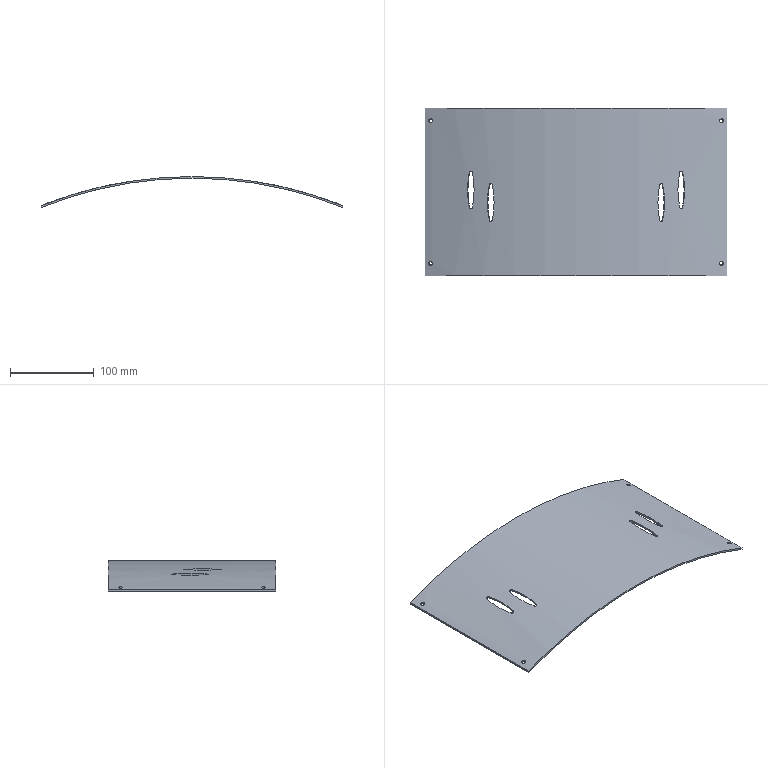Part | STEP file | 1 solid | 26 faces | box 360 x 200 x 36.871 mm | volume 145158 mm3 | cylinder 22 | plane 4 | commonest cylinder face diameters 3.8 x8 204.176 x8 4.6 x4 964 x1 968 x1